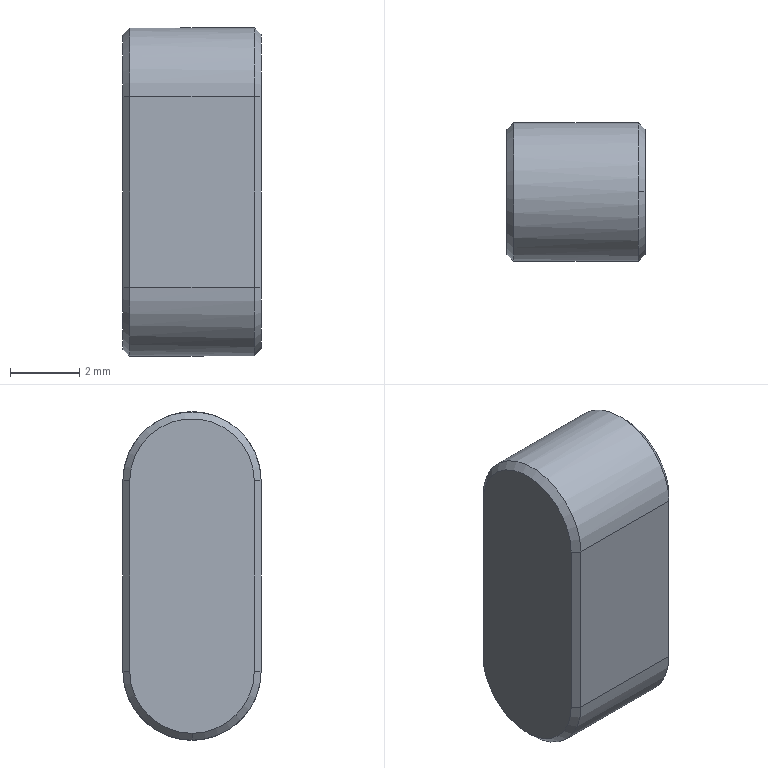Part | STEP file | 02-08 Driving sprocket key | 1 solid | 16 faces | box 4 x 4 x 9.5 mm | volume 137.34 mm3 | plane 8 | cone 6 | cylinder 2 | commonest cylinder face diameters 4 x2
STEP:
#1=CARTESIAN_POINT('',(0.,0.,0.));
#2=DIRECTION('',(0.,0.,1.));
#3=DIRECTION('',(1.,0.,0.));
#4=AXIS2_PLACEMENT_3D('',#1,#2,#3);
#5=CARTESIAN_POINT('',(4.,0.,1.8));
#6=VERTEX_POINT('',#5);
#7=CARTESIAN_POINT('',(4.,-1.8,0.));
#8=VERTEX_POINT('',#7);
#9=CARTESIAN_POINT('',(4.,0.,0.));
#10=DIRECTION('',(1.,0.,0.));
#11=DIRECTION('',(0.,0.,1.));
#12=AXIS2_PLACEMENT_3D('',#9,#10,#11);
#13=CIRCLE('',#12,1.8);
#14=CARTESIAN_POINT('',(4.,0.,0.));
#15=DIRECTION('',(-1.,0.,0.));
#16=DIRECTION('',(0.,0.,1.));
#17=AXIS2_PLACEMENT_3D('',#14,#15,#16);
#18=CONICAL_SURFACE('',#17,1.8,0.7854);
#19=CARTESIAN_POINT('',(6.283,0.));
#20=DIRECTION('',(-1.,0.));
#21=VECTOR('',#20,1.);
#22=LINE('',#19,#21);
#23=(GEOMETRIC_REPRESENTATION_CONTEXT(2)PARAMETRIC_REPRESENTATION_CONTEXT()REPRESENTATION_CONTEXT('',''));
#24=DEFINITIONAL_REPRESENTATION('',(#22),#23);
#25=PCURVE('',#18,#24);
#26=CARTESIAN_POINT('',(4.,-1.8,1.855));
#27=DIRECTION('',(1.,0.,0.));
#28=DIRECTION('',(0.,0.,-1.));
#29=AXIS2_PLACEMENT_3D('',#26,#27,#28);
#30=PLANE('',#29);
#31=CARTESIAN_POINT('',(1.855,1.8));
#32=DIRECTION('',(-1.,0.));
#33=AXIS2_PLACEMENT_2D('',#31,#32);
#34=CIRCLE('',#33,1.8);
#35=(GEOMETRIC_REPRESENTATION_CONTEXT(2)PARAMETRIC_REPRESENTATION_CONTEXT()REPRESENTATION_CONTEXT('',''));
#36=DEFINITIONAL_REPRESENTATION('',(#34),#35);
#37=PCURVE('',#30,#36);
#38=SURFACE_CURVE('',#13,(#25,#37),.PCURVE_S1.);
#39=EDGE_CURVE('',#6,#8,#38,.T.);
#40=ORIENTED_EDGE('',*,*,#39,.F.);
#41=CARTESIAN_POINT('',(3.8,0.,2.));
#42=VERTEX_POINT('',#41);
#43=CARTESIAN_POINT('',(4.,0.,1.8));
#44=DIRECTION('',(-0.7071,0.,0.7071));
#45=VECTOR('',#44,1.);
#46=LINE('',#43,#45);
#47=CARTESIAN_POINT('',(6.283,0.));
#48=DIRECTION('',(0.,1.));
#49=VECTOR('',#48,1.);
#50=LINE('',#47,#49);
#51=(GEOMETRIC_REPRESENTATION_CONTEXT(2)PARAMETRIC_REPRESENTATION_CONTEXT()REPRESENTATION_CONTEXT('',''));
#52=DEFINITIONAL_REPRESENTATION('',(#50),#51);
#53=PCURVE('',#18,#52);
#54=CARTESIAN_POINT('',(4.,0.,0.));
#55=DIRECTION('',(-1.,0.,0.));
#56=DIRECTION('',(0.,0.,1.));
#57=AXIS2_PLACEMENT_3D('',#54,#55,#56);
#58=CONICAL_SURFACE('',#57,1.8,0.7854);
#59=CARTESIAN_POINT('',(0.,0.));
#60=DIRECTION('',(0.,1.));
#61=VECTOR('',#60,1.);
#62=LINE('',#59,#61);
#63=(GEOMETRIC_REPRESENTATION_CONTEXT(2)PARAMETRIC_REPRESENTATION_CONTEXT()REPRESENTATION_CONTEXT('',''));
#64=DEFINITIONAL_REPRESENTATION('',(#62),#63);
#65=PCURVE('',#58,#64);
#66=SURFACE_CURVE('',#46,(#53,#65),.PCURVE_S1.);
#67=EDGE_CURVE('',#6,#42,#66,.T.);
#68=ORIENTED_EDGE('',*,*,#67,.T.);
#69=CARTESIAN_POINT('',(3.8,-2.,0.));
#70=VERTEX_POINT('',#69);
#71=CARTESIAN_POINT('',(3.8,0.,0.));
#72=DIRECTION('',(-1.,0.,0.));
#73=DIRECTION('',(0.,0.,1.));
#74=AXIS2_PLACEMENT_3D('',#71,#72,#73);
#75=CIRCLE('',#74,2.);
#76=CARTESIAN_POINT('',(0.,0.2));
#77=DIRECTION('',(1.,0.));
#78=VECTOR('',#77,1.);
#79=LINE('',#76,#78);
#80=(GEOMETRIC_REPRESENTATION_CONTEXT(2)PARAMETRIC_REPRESENTATION_CONTEXT()REPRESENTATION_CONTEXT('',''));
#81=DEFINITIONAL_REPRESENTATION('',(#79),#80);
#82=PCURVE('',#18,#81);
#83=CARTESIAN_POINT('',(3.8,0.,0.));
#84=DIRECTION('',(-1.,0.,0.));
#85=DIRECTION('',(0.,-1.,0.));
#86=AXIS2_PLACEMENT_3D('',#83,#84,#85);
#87=CYLINDRICAL_SURFACE('',#86,2.);
#88=CARTESIAN_POINT('',(-4.712,0.));
#89=DIRECTION('',(1.,0.));
#90=VECTOR('',#89,1.);
#91=LINE('',#88,#90);
#92=(GEOMETRIC_REPRESENTATION_CONTEXT(2)PARAMETRIC_REPRESENTATION_CONTEXT()REPRESENTATION_CONTEXT('',''));
#93=DEFINITIONAL_REPRESENTATION('',(#91),#92);
#94=PCURVE('',#87,#93);
#95=SURFACE_CURVE('',#75,(#82,#94),.PCURVE_S1.);
#96=EDGE_CURVE('',#70,#42,#95,.T.);
#97=ORIENTED_EDGE('',*,*,#96,.F.);
#98=CARTESIAN_POINT('',(3.9,-1.9,0.));
#99=DIRECTION('',(-0.7071,-0.7071,0.));
#100=VECTOR('',#99,1.);
#101=LINE('',#98,#100);
#102=CARTESIAN_POINT('',(4.712,0.1));
#103=DIRECTION('',(0.,1.));
#104=VECTOR('',#103,1.);
#105=LINE('',#102,#104);
#106=(GEOMETRIC_REPRESENTATION_CONTEXT(2)PARAMETRIC_REPRESENTATION_CONTEXT()REPRESENTATION_CONTEXT('',''));
#107=DEFINITIONAL_REPRESENTATION('',(#105),#106);
#108=PCURVE('',#18,#107);
#109=CARTESIAN_POINT('',(3.8,-2.,-5.5));
#110=DIRECTION('',(0.7071,-0.7071,0.));
#111=DIRECTION('',(0.7071,0.7071,0.));
#112=AXIS2_PLACEMENT_3D('',#109,#110,#111);
#113=PLANE('',#112);
#114=CARTESIAN_POINT('',(0.1414,5.5));
#115=DIRECTION('',(-1.,0.));
#116=VECTOR('',#115,1.);
#117=LINE('',#114,#116);
#118=(GEOMETRIC_REPRESENTATION_CONTEXT(2)PARAMETRIC_REPRESENTATION_CONTEXT()REPRESENTATION_CONTEXT('',''));
#119=DEFINITIONAL_REPRESENTATION('',(#117),#118);
#120=PCURVE('',#113,#119);
#121=SURFACE_CURVE('',#101,(#108,#120),.PCURVE_S1.);
#122=EDGE_CURVE('',#8,#70,#121,.T.);
#123=ORIENTED_EDGE('',*,*,#122,.F.);
#124=EDGE_LOOP('',(#40,#68,#97,#123));
#125=FACE_BOUND('',#124,.T.);
#126=ADVANCED_FACE('',(#125),#18,.T.);
#127=CARTESIAN_POINT('',(0.,-1.8,-5.5));
#128=VERTEX_POINT('',#127);
#129=CARTESIAN_POINT('',(0.,0.,-7.3));
#130=VERTEX_POINT('',#129);
#131=CARTESIAN_POINT('',(0.,0.,-5.5));
#132=DIRECTION('',(1.,0.,0.));
#133=DIRECTION('',(0.,0.,-1.));
#134=AXIS2_PLACEMENT_3D('',#131,#132,#133);
#135=CIRCLE('',#134,1.8);
#136=CARTESIAN_POINT('',(0.,0.,-5.5));
#137=DIRECTION('',(1.,0.,0.));
#138=DIRECTION('',(0.,0.,-1.));
#139=AXIS2_PLACEMENT_3D('',#136,#137,#138);
#140=CONICAL_SURFACE('',#139,1.8,0.7854);
#141=CARTESIAN_POINT('',(0.,0.));
#142=DIRECTION('',(1.,0.));
#143=VECTOR('',#142,1.);
#144=LINE('',#141,#143);
#145=(GEOMETRIC_REPRESENTATION_CONTEXT(2)PARAMETRIC_REPRESENTATION_CONTEXT()REPRESENTATION_CONTEXT('',''));
#146=DEFINITIONAL_REPRESENTATION('',(#144),#145);
#147=PCURVE('',#140,#146);
#148=CARTESIAN_POINT('',(0.,-1.8,1.855));
#149=DIRECTION('',(1.,0.,0.));
#150=DIRECTION('',(0.,0.,-1.));
#151=AXIS2_PLACEMENT_3D('',#148,#149,#150);
#152=PLANE('',#151);
#153=CARTESIAN_POINT('',(7.355,1.8));
#154=DIRECTION('',(1.,0.));
#155=AXIS2_PLACEMENT_2D('',#153,#154);
#156=CIRCLE('',#155,1.8);
#157=(GEOMETRIC_REPRESENTATION_CONTEXT(2)PARAMETRIC_REPRESENTATION_CONTEXT()REPRESENTATION_CONTEXT('',''));
#158=DEFINITIONAL_REPRESENTATION('',(#156),#157);
#159=PCURVE('',#152,#158);
#160=SURFACE_CURVE('',#135,(#147,#159),.PCURVE_S1.);
#161=EDGE_CURVE('',#128,#130,#160,.T.);
#162=ORIENTED_EDGE('',*,*,#161,.T.);
#163=CARTESIAN_POINT('',(0.2,0.,-7.5));
#164=VERTEX_POINT('',#163);
#165=CARTESIAN_POINT('',(0.,0.,-7.3));
#166=DIRECTION('',(0.7071,0.,-0.7071));
#167=VECTOR('',#166,1.);
#168=LINE('',#165,#167);
#169=CARTESIAN_POINT('',(6.283,0.));
#170=DIRECTION('',(0.,1.));
#171=VECTOR('',#170,1.);
#172=LINE('',#169,#171);
#173=(GEOMETRIC_REPRESENTATION_CONTEXT(2)PARAMETRIC_REPRESENTATION_CONTEXT()REPRESENTATION_CONTEXT('',''));
#174=DEFINITIONAL_REPRESENTATION('',(#172),#173);
#175=PCURVE('',#140,#174);
#176=CARTESIAN_POINT('',(0.,0.,-5.5));
#177=DIRECTION('',(1.,0.,0.));
#178=DIRECTION('',(0.,0.,-1.));
#179=AXIS2_PLACEMENT_3D('',#176,#177,#178);
#180=CONICAL_SURFACE('',#179,1.8,0.7854);
#181=CARTESIAN_POINT('',(0.,0.));
#182=DIRECTION('',(0.,1.));
#183=VECTOR('',#182,1.);
#184=LINE('',#181,#183);
#185=(GEOMETRIC_REPRESENTATION_CONTEXT(2)PARAMETRIC_REPRESENTATION_CONTEXT()REPRESENTATION_CONTEXT('',''));
#186=DEFINITIONAL_REPRESENTATION('',(#184),#185);
#187=PCURVE('',#180,#186);
#188=SURFACE_CURVE('',#168,(#175,#187),.PCURVE_S1.);
#189=EDGE_CURVE('',#130,#164,#188,.T.);
#190=ORIENTED_EDGE('',*,*,#189,.T.);
#191=CARTESIAN_POINT('',(0.2,-2.,-5.5));
#192=VERTEX_POINT('',#191);
#193=CARTESIAN_POINT('',(0.2,0.,-5.5));
#194=DIRECTION('',(-1.,0.,0.));
#195=DIRECTION('',(0.,0.,1.));
#196=AXIS2_PLACEMENT_3D('',#193,#194,#195);
#197=CIRCLE('',#196,2.);
#198=CARTESIAN_POINT('',(9.425,0.2));
#199=DIRECTION('',(-1.,0.));
#200=VECTOR('',#199,1.);
#201=LINE('',#198,#200);
#202=(GEOMETRIC_REPRESENTATION_CONTEXT(2)PARAMETRIC_REPRESENTATION_CONTEXT()REPRESENTATION_CONTEXT('',''));
#203=DEFINITIONAL_REPRESENTATION('',(#201),#202);
#204=PCURVE('',#140,#203);
#205=CARTESIAN_POINT('',(3.8,0.,-5.5));
#206=DIRECTION('',(-1.,0.,0.));
#207=DIRECTION('',(0.,-1.,0.));
#208=AXIS2_PLACEMENT_3D('',#205,#206,#207);
#209=CYLINDRICAL_SURFACE('',#208,2.);
#210=CARTESIAN_POINT('',(1.571,3.6));
#211=DIRECTION('',(1.,0.));
#212=VECTOR('',#211,1.);
#213=LINE('',#210,#212);
#214=(GEOMETRIC_REPRESENTATION_CONTEXT(2)PARAMETRIC_REPRESENTATION_CONTEXT()REPRESENTATION_CONTEXT('',''));
#215=DEFINITIONAL_REPRESENTATION('',(#213),#214);
#216=PCURVE('',#209,#215);
#217=SURFACE_CURVE('',#197,(#204,#216),.PCURVE_S1.);
#218=EDGE_CURVE('',#164,#192,#217,.T.);
#219=ORIENTED_EDGE('',*,*,#218,.T.);
#220=CARTESIAN_POINT('',(0.1,-1.9,-5.5));
#221=DIRECTION('',(-0.7071,0.7071,0.));
#222=VECTOR('',#221,1.);
#223=LINE('',#220,#222);
#224=CARTESIAN_POINT('',(4.712,0.1));
#225=DIRECTION('',(0.,-1.));
#226=VECTOR('',#225,1.);
#227=LINE('',#224,#226);
#228=(GEOMETRIC_REPRESENTATION_CONTEXT(2)PARAMETRIC_REPRESENTATION_CONTEXT()REPRESENTATION_CONTEXT('',''));
#229=DEFINITIONAL_REPRESENTATION('',(#227),#228);
#230=PCURVE('',#140,#229);
#231=CARTESIAN_POINT('',(0.2,-2.,-5.5));
#232=DIRECTION('',(0.7071,0.7071,0.));
#233=DIRECTION('',(-0.7071,0.7071,0.));
#234=AXIS2_PLACEMENT_3D('',#231,#232,#233);
#235=PLANE('',#234);
#236=CARTESIAN_POINT('',(0.1414,0.));
#237=DIRECTION('',(1.,0.));
#238=VECTOR('',#237,1.);
#239=LINE('',#236,#238);
#240=(GEOMETRIC_REPRESENTATION_CONTEXT(2)PARAMETRIC_REPRESENTATION_CONTEXT()REPRESENTATION_CONTEXT('',''));
#241=DEFINITIONAL_REPRESENTATION('',(#239),#240);
#242=PCURVE('',#235,#241);
#243=SURFACE_CURVE('',#223,(#230,#242),.PCURVE_S1.);
#244=EDGE_CURVE('',#192,#128,#243,.T.);
#245=ORIENTED_EDGE('',*,*,#244,.T.);
#246=EDGE_LOOP('',(#162,#190,#219,#245));
#247=FACE_BOUND('',#246,.T.);
#248=ADVANCED_FACE('',(#247),#140,.T.);
#249=ORIENTED_EDGE('',*,*,#67,.F.);
#250=CARTESIAN_POINT('',(4.,1.8,0.));
#251=VERTEX_POINT('',#250);
#252=CARTESIAN_POINT('',(4.,0.,0.));
#253=DIRECTION('',(1.,0.,0.));
#254=DIRECTION('',(0.,0.,1.));
#255=AXIS2_PLACEMENT_3D('',#252,#253,#254);
#256=CIRCLE('',#255,1.8);
#257=CARTESIAN_POINT('',(6.283,0.));
#258=DIRECTION('',(-1.,0.));
#259=VECTOR('',#258,1.);
#260=LINE('',#257,#259);
#261=(GEOMETRIC_REPRESENTATION_CONTEXT(2)PARAMETRIC_REPRESENTATION_CONTEXT()REPRESENTATION_CONTEXT('',''));
#262=DEFINITIONAL_REPRESENTATION('',(#260),#261);
#263=PCURVE('',#58,#262);
#264=CARTESIAN_POINT('',(1.855,1.8));
#265=DIRECTION('',(-1.,0.));
#266=AXIS2_PLACEMENT_2D('',#264,#265);
#267=CIRCLE('',#266,1.8);
#268=(GEOMETRIC_REPRESENTATION_CONTEXT(2)PARAMETRIC_REPRESENTATION_CONTEXT()REPRESENTATION_CONTEXT('',''));
#269=DEFINITIONAL_REPRESENTATION('',(#267),#268);
#270=PCURVE('',#30,#269);
#271=SURFACE_CURVE('',#256,(#263,#270),.PCURVE_S1.);
#272=EDGE_CURVE('',#251,#6,#271,.T.);
#273=ORIENTED_EDGE('',*,*,#272,.F.);
#274=CARTESIAN_POINT('',(3.8,2.,0.));
#275=VERTEX_POINT('',#274);
#276=CARTESIAN_POINT('',(3.9,1.9,0.));
#277=DIRECTION('',(0.7071,-0.7071,0.));
#278=VECTOR('',#277,1.);
#279=LINE('',#276,#278);
#280=CARTESIAN_POINT('',(1.571,0.1));
#281=DIRECTION('',(0.,-1.));
#282=VECTOR('',#281,1.);
#283=LINE('',#280,#282);
#284=(GEOMETRIC_REPRESENTATION_CONTEXT(2)PARAMETRIC_REPRESENTATION_CONTEXT()REPRESENTATION_CONTEXT('',''));
#285=DEFINITIONAL_REPRESENTATION('',(#283),#284);
#286=PCURVE('',#58,#285);
#287=CARTESIAN_POINT('',(4.,1.8,-5.5));
#288=DIRECTION('',(0.7071,0.7071,0.));
#289=DIRECTION('',(-0.7071,0.7071,0.));
#290=AXIS2_PLACEMENT_3D('',#287,#288,#289);
#291=PLANE('',#290);
#292=CARTESIAN_POINT('',(0.1414,5.5));
#293=DIRECTION('',(-1.,0.));
#294=VECTOR('',#293,1.);
#295=LINE('',#292,#294);
#296=(GEOMETRIC_REPRESENTATION_CONTEXT(2)PARAMETRIC_REPRESENTATION_CONTEXT()REPRESENTATION_CONTEXT('',''));
#297=DEFINITIONAL_REPRESENTATION('',(#295),#296);
#298=PCURVE('',#291,#297);
#299=SURFACE_CURVE('',#279,(#286,#298),.PCURVE_S1.);
#300=EDGE_CURVE('',#275,#251,#299,.T.);
#301=ORIENTED_EDGE('',*,*,#300,.F.);
#302=CARTESIAN_POINT('',(3.8,0.,0.));
#303=DIRECTION('',(-1.,0.,0.));
#304=DIRECTION('',(0.,0.,1.));
#305=AXIS2_PLACEMENT_3D('',#302,#303,#304);
#306=CIRCLE('',#305,2.);
#307=CARTESIAN_POINT('',(0.,0.2));
#308=DIRECTION('',(1.,0.));
#309=VECTOR('',#308,1.);
#310=LINE('',#307,#309);
#311=(GEOMETRIC_REPRESENTATION_CONTEXT(2)PARAMETRIC_REPRESENTATION_CONTEXT()REPRESENTATION_CONTEXT('',''));
#312=DEFINITIONAL_REPRESENTATION('',(#310),#311);
#313=PCURVE('',#58,#312);
#314=CARTESIAN_POINT('',(1.571,0.));
#315=DIRECTION('',(1.,0.));
#316=VECTOR('',#315,1.);
#317=LINE('',#314,#316);
#318=(GEOMETRIC_REPRESENTATION_CONTEXT(2)PARAMETRIC_REPRESENTATION_CONTEXT()REPRESENTATION_CONTEXT('',''));
#319=DEFINITIONAL_REPRESENTATION('',(#317),#318);
#320=PCURVE('',#87,#319);
#321=SURFACE_CURVE('',#306,(#313,#320),.PCURVE_S1.);
#322=EDGE_CURVE('',#42,#275,#321,.T.);
#323=ORIENTED_EDGE('',*,*,#322,.F.);
#324=EDGE_LOOP('',(#249,#273,#301,#323));
#325=FACE_BOUND('',#324,.T.);
#326=ADVANCED_FACE('',(#325),#58,.T.);
#327=CARTESIAN_POINT('',(4.,-1.8,-5.5));
#328=VERTEX_POINT('',#327);
#329=CARTESIAN_POINT('',(4.,1.8,-5.5));
#330=VERTEX_POINT('',#329);
#331=CARTESIAN_POINT('',(4.,0.,-5.5));
#332=DIRECTION('',(1.,0.,0.));
#333=DIRECTION('',(0.,0.,1.));
#334=AXIS2_PLACEMENT_3D('',#331,#332,#333);
#335=CIRCLE('',#334,1.8);
#336=CARTESIAN_POINT('',(7.355,1.8));
#337=DIRECTION('',(-1.,0.));
#338=AXIS2_PLACEMENT_2D('',#336,#337);
#339=CIRCLE('',#338,1.8);
#340=(GEOMETRIC_REPRESENTATION_CONTEXT(2)PARAMETRIC_REPRESENTATION_CONTEXT()REPRESENTATION_CONTEXT('',''));
#341=DEFINITIONAL_REPRESENTATION('',(#339),#340);
#342=PCURVE('',#30,#341);
#343=CARTESIAN_POINT('',(4.,0.,-5.5));
#344=DIRECTION('',(-1.,0.,0.));
#345=DIRECTION('',(0.,0.,1.));
#346=AXIS2_PLACEMENT_3D('',#343,#344,#345);
#347=CONICAL_SURFACE('',#346,1.8,0.7854);
#348=CARTESIAN_POINT('',(6.283,0.));
#349=DIRECTION('',(-1.,0.));
#350=VECTOR('',#349,1.);
#351=LINE('',#348,#350);
#352=(GEOMETRIC_REPRESENTATION_CONTEXT(2)PARAMETRIC_REPRESENTATION_CONTEXT()REPRESENTATION_CONTEXT('',''));
#353=DEFINITIONAL_REPRESENTATION('',(#351),#352);
#354=PCURVE('',#347,#353);
#355=SURFACE_CURVE('',#335,(#342,#354),.PCURVE_S1.);
#356=EDGE_CURVE('',#328,#330,#355,.T.);
#357=ORIENTED_EDGE('',*,*,#356,.T.);
#358=CARTESIAN_POINT('',(4.,1.8,-2.75));
#359=DIRECTION('',(0.,0.,1.));
#360=VECTOR('',#359,1.);
#361=LINE('',#358,#360);
#362=CARTESIAN_POINT('',(4.605,3.6));
#363=DIRECTION('',(-1.,0.));
#364=VECTOR('',#363,1.);
#365=LINE('',#362,#364);
#366=(GEOMETRIC_REPRESENTATION_CONTEXT(2)PARAMETRIC_REPRESENTATION_CONTEXT()REPRESENTATION_CONTEXT('',''));
#367=DEFINITIONAL_REPRESENTATION('',(#365),#366);
#368=PCURVE('',#30,#367);
#369=CARTESIAN_POINT('',(0.,2.75));
#370=DIRECTION('',(0.,1.));
#371=VECTOR('',#370,1.);
#372=LINE('',#369,#371);
#373=(GEOMETRIC_REPRESENTATION_CONTEXT(2)PARAMETRIC_REPRESENTATION_CONTEXT()REPRESENTATION_CONTEXT('',''));
#374=DEFINITIONAL_REPRESENTATION('',(#372),#373);
#375=PCURVE('',#291,#374);
#376=SURFACE_CURVE('',#361,(#368,#375),.PCURVE_S1.);
#377=EDGE_CURVE('',#330,#251,#376,.T.);
#378=ORIENTED_EDGE('',*,*,#377,.T.);
#379=ORIENTED_EDGE('',*,*,#272,.T.);
#380=ORIENTED_EDGE('',*,*,#39,.T.);
#381=CARTESIAN_POINT('',(4.,-1.8,-2.75));
#382=DIRECTION('',(0.,0.,-1.));
#383=VECTOR('',#382,1.);
#384=LINE('',#381,#383);
#385=CARTESIAN_POINT('',(4.605,0.));
#386=DIRECTION('',(1.,0.));
#387=VECTOR('',#386,1.);
#388=LINE('',#385,#387);
#389=(GEOMETRIC_REPRESENTATION_CONTEXT(2)PARAMETRIC_REPRESENTATION_CONTEXT()REPRESENTATION_CONTEXT('',''));
#390=DEFINITIONAL_REPRESENTATION('',(#388),#389);
#391=PCURVE('',#30,#390);
#392=CARTESIAN_POINT('',(0.2828,2.75));
#393=DIRECTION('',(0.,-1.));
#394=VECTOR('',#393,1.);
#395=LINE('',#392,#394);
#396=(GEOMETRIC_REPRESENTATION_CONTEXT(2)PARAMETRIC_REPRESENTATION_CONTEXT()REPRESENTATION_CONTEXT('',''));
#397=DEFINITIONAL_REPRESENTATION('',(#395),#396);
#398=PCURVE('',#113,#397);
#399=SURFACE_CURVE('',#384,(#391,#398),.PCURVE_S1.);
#400=EDGE_CURVE('',#8,#328,#399,.T.);
#401=ORIENTED_EDGE('',*,*,#400,.T.);
#402=EDGE_LOOP('',(#357,#378,#379,#380,#401));
#403=FACE_BOUND('',#402,.T.);
#404=ADVANCED_FACE('',(#403),#30,.T.);
#405=ORIENTED_EDGE('',*,*,#96,.T.);
#406=ORIENTED_EDGE('',*,*,#322,.T.);
#407=CARTESIAN_POINT('',(0.2,2.,0.));
#408=VERTEX_POINT('',#407);
#409=CARTESIAN_POINT('',(2.,2.,0.));
#410=DIRECTION('',(1.,0.,0.));
#411=VECTOR('',#410,1.);
#412=LINE('',#409,#411);
#413=CARTESIAN_POINT('',(3.142,1.8));
#414=DIRECTION('',(0.,-1.));
#415=VECTOR('',#414,1.);
#416=LINE('',#413,#415);
#417=(GEOMETRIC_REPRESENTATION_CONTEXT(2)PARAMETRIC_REPRESENTATION_CONTEXT()REPRESENTATION_CONTEXT('',''));
#418=DEFINITIONAL_REPRESENTATION('',(#416),#417);
#419=PCURVE('',#87,#418);
#420=CARTESIAN_POINT('',(0.2,2.,0.));
#421=DIRECTION('',(0.,-1.,0.));
#422=DIRECTION('',(0.,0.,-1.));
#423=AXIS2_PLACEMENT_3D('',#420,#421,#422);
#424=PLANE('',#423);
#425=CARTESIAN_POINT('',(0.,1.8));
#426=DIRECTION('',(0.,1.));
#427=VECTOR('',#426,1.);
#428=LINE('',#425,#427);
#429=(GEOMETRIC_REPRESENTATION_CONTEXT(2)PARAMETRIC_REPRESENTATION_CONTEXT()REPRESENTATION_CONTEXT('',''));
#430=DEFINITIONAL_REPRESENTATION('',(#428),#429);
#431=PCURVE('',#424,#430);
#432=SURFACE_CURVE('',#412,(#419,#431),.PCURVE_S1.);
#433=EDGE_CURVE('',#408,#275,#432,.T.);
#434=ORIENTED_EDGE('',*,*,#433,.F.);
#435=CARTESIAN_POINT('',(0.2,-2.,0.));
#436=VERTEX_POINT('',#435);
#437=CARTESIAN_POINT('',(0.2,0.,0.));
#438=DIRECTION('',(-1.,0.,0.));
#439=DIRECTION('',(0.,0.,1.));
#440=AXIS2_PLACEMENT_3D('',#437,#438,#439);
#441=CIRCLE('',#440,2.);
#442=CARTESIAN_POINT('',(-4.712,3.6));
#443=DIRECTION('',(1.,0.));
#444=VECTOR('',#443,1.);
#445=LINE('',#442,#444);
#446=(GEOMETRIC_REPRESENTATION_CONTEXT(2)PARAMETRIC_REPRESENTATION_CONTEXT()REPRESENTATION_CONTEXT('',''));
#447=DEFINITIONAL_REPRESENTATION('',(#445),#446);
#448=PCURVE('',#87,#447);
#449=CARTESIAN_POINT('',(0.,0.,0.));
#450=DIRECTION('',(1.,0.,0.));
#451=DIRECTION('',(0.,0.,-1.));
#452=AXIS2_PLACEMENT_3D('',#449,#450,#451);
#453=CONICAL_SURFACE('',#452,1.8,0.7854);
#454=CARTESIAN_POINT('',(9.425,0.2));
#455=DIRECTION('',(-1.,0.));
#456=VECTOR('',#455,1.);
#457=LINE('',#454,#456);
#458=(GEOMETRIC_REPRESENTATION_CONTEXT(2)PARAMETRIC_REPRESENTATION_CONTEXT()REPRESENTATION_CONTEXT('',''));
#459=DEFINITIONAL_REPRESENTATION('',(#457),#458);
#460=PCURVE('',#453,#459);
#461=SURFACE_CURVE('',#441,(#448,#460),.PCURVE_S1.);
#462=EDGE_CURVE('',#436,#408,#461,.T.);
#463=ORIENTED_EDGE('',*,*,#462,.F.);
#464=CARTESIAN_POINT('',(2.,-2.,-0.000000001));
#465=DIRECTION('',(-1.,0.,0.));
#466=VECTOR('',#465,1.);
#467=LINE('',#464,#466);
#468=CARTESIAN_POINT('',(0.,1.8));
#469=DIRECTION('',(0.,1.));
#470=VECTOR('',#469,1.);
#471=LINE('',#468,#470);
#472=(GEOMETRIC_REPRESENTATION_CONTEXT(2)PARAMETRIC_REPRESENTATION_CONTEXT()REPRESENTATION_CONTEXT('',''));
#473=DEFINITIONAL_REPRESENTATION('',(#471),#472);
#474=PCURVE('',#87,#473);
#475=CARTESIAN_POINT('',(0.2,-2.,-5.5));
#476=DIRECTION('',(0.,1.,0.));
#477=DIRECTION('',(0.,0.,1.));
#478=AXIS2_PLACEMENT_3D('',#475,#476,#477);
#479=PLANE('',#478);
#480=CARTESIAN_POINT('',(5.5,1.8));
#481=DIRECTION('',(0.,-1.));
#482=VECTOR('',#481,1.);
#483=LINE('',#480,#482);
#484=(GEOMETRIC_REPRESENTATION_CONTEXT(2)PARAMETRIC_REPRESENTATION_CONTEXT()REPRESENTATION_CONTEXT('',''));
#485=DEFINITIONAL_REPRESENTATION('',(#483),#484);
#486=PCURVE('',#479,#485);
#487=SURFACE_CURVE('',#467,(#474,#486),.PCURVE_S1.);
#488=EDGE_CURVE('',#70,#436,#487,.T.);
#489=ORIENTED_EDGE('',*,*,#488,.F.);
#490=EDGE_LOOP('',(#405,#406,#434,#463,#489));
#491=FACE_BOUND('',#490,.T.);
#492=ADVANCED_FACE('',(#491),#87,.T.);
#493=ORIENTED_EDGE('',*,*,#300,.T.);
#494=ORIENTED_EDGE('',*,*,#377,.F.);
#495=CARTESIAN_POINT('',(3.8,2.,-5.5));
#496=VERTEX_POINT('',#495);
#497=CARTESIAN_POINT('',(3.9,1.9,-5.5));
#498=DIRECTION('',(-0.7071,0.7071,0.));
#499=VECTOR('',#498,1.);
#500=LINE('',#497,#499);
#501=CARTESIAN_POINT('',(0.1414,0.));
#502=DIRECTION('',(1.,0.));
#503=VECTOR('',#502,1.);
#504=LINE('',#501,#503);
#505=(GEOMETRIC_REPRESENTATION_CONTEXT(2)PARAMETRIC_REPRESENTATION_CONTEXT()REPRESENTATION_CONTEXT('',''));
#506=DEFINITIONAL_REPRESENTATION('',(#504),#505);
#507=PCURVE('',#291,#506);
#508=CARTESIAN_POINT('',(1.571,0.1));
#509=DIRECTION('',(0.,1.));
#510=VECTOR('',#509,1.);
#511=LINE('',#508,#510);
#512=(GEOMETRIC_REPRESENTATION_CONTEXT(2)PARAMETRIC_REPRESENTATION_CONTEXT()REPRESENTATION_CONTEXT('',''));
#513=DEFINITIONAL_REPRESENTATION('',(#511),#512);
#514=PCURVE('',#347,#513);
#515=SURFACE_CURVE('',#500,(#507,#514),.PCURVE_S1.);
#516=EDGE_CURVE('',#330,#496,#515,.T.);
#517=ORIENTED_EDGE('',*,*,#516,.T.);
#518=CARTESIAN_POINT('',(3.8,2.,-2.75));
#519=DIRECTION('',(0.,0.,1.));
#520=VECTOR('',#519,1.);
#521=LINE('',#518,#520);
#522=CARTESIAN_POINT('',(0.2828,2.75));
#523=DIRECTION('',(0.,1.));
#524=VECTOR('',#523,1.);
#525=LINE('',#522,#524);
#526=(GEOMETRIC_REPRESENTATION_CONTEXT(2)PARAMETRIC_REPRESENTATION_CONTEXT()REPRESENTATION_CONTEXT('',''));
#527=DEFINITIONAL_REPRESENTATION('',(#525),#526);
#528=PCURVE('',#291,#527);
#529=CARTESIAN_POINT('',(2.75,3.6));
#530=DIRECTION('',(-1.,0.));
#531=VECTOR('',#530,1.);
#532=LINE('',#529,#531);
#533=(GEOMETRIC_REPRESENTATION_CONTEXT(2)PARAMETRIC_REPRESENTATION_CONTEXT()REPRESENTATION_CONTEXT('',''));
#534=DEFINITIONAL_REPRESENTATION('',(#532),#533);
#535=PCURVE('',#424,#534);
#536=SURFACE_CURVE('',#521,(#528,#535),.PCURVE_S1.);
#537=EDGE_CURVE('',#496,#275,#536,.T.);
#538=ORIENTED_EDGE('',*,*,#537,.T.);
#539=EDGE_LOOP('',(#493,#494,#517,#538));
#540=FACE_BOUND('',#539,.T.);
#541=ADVANCED_FACE('',(#540),#291,.T.);
#542=ORIENTED_EDGE('',*,*,#356,.F.);
#543=CARTESIAN_POINT('',(3.8,-2.,-5.5));
#544=VERTEX_POINT('',#543);
#545=CARTESIAN_POINT('',(3.9,-1.9,-5.5));
#546=DIRECTION('',(0.7071,0.7071,0.));
#547=VECTOR('',#546,1.);
#548=LINE('',#545,#547);
#549=CARTESIAN_POINT('',(4.712,0.1));
#550=DIRECTION('',(0.,-1.));
#551=VECTOR('',#550,1.);
#552=LINE('',#549,#551);
#553=(GEOMETRIC_REPRESENTATION_CONTEXT(2)PARAMETRIC_REPRESENTATION_CONTEXT()REPRESENTATION_CONTEXT('',''));
#554=DEFINITIONAL_REPRESENTATION('',(#552),#553);
#555=PCURVE('',#347,#554);
#556=CARTESIAN_POINT('',(0.1414,-0.000000001));
#557=DIRECTION('',(1.,0.));
#558=VECTOR('',#557,1.);
#559=LINE('',#556,#558);
#560=(GEOMETRIC_REPRESENTATION_CONTEXT(2)PARAMETRIC_REPRESENTATION_CONTEXT()REPRESENTATION_CONTEXT('',''));
#561=DEFINITIONAL_REPRESENTATION('',(#559),#560);
#562=PCURVE('',#113,#561);
#563=SURFACE_CURVE('',#548,(#555,#562),.PCURVE_S1.);
#564=EDGE_CURVE('',#544,#328,#563,.T.);
#565=ORIENTED_EDGE('',*,*,#564,.F.);
#566=CARTESIAN_POINT('',(3.8,0.,-5.5));
#567=DIRECTION('',(-1.,0.,0.));
#568=DIRECTION('',(0.,0.,1.));
#569=AXIS2_PLACEMENT_3D('',#566,#567,#568);
#570=CIRCLE('',#569,2.);
#571=CARTESIAN_POINT('',(0.,0.2));
#572=DIRECTION('',(1.,0.));
#573=VECTOR('',#572,1.);
#574=LINE('',#571,#573);
#575=(GEOMETRIC_REPRESENTATION_CONTEXT(2)PARAMETRIC_REPRESENTATION_CONTEXT()REPRESENTATION_CONTEXT('',''));
#576=DEFINITIONAL_REPRESENTATION('',(#574),#575);
#577=PCURVE('',#347,#576);
#578=CARTESIAN_POINT('',(1.571,0.));
#579=DIRECTION('',(1.,0.));
#580=VECTOR('',#579,1.);
#581=LINE('',#578,#580);
#582=(GEOMETRIC_REPRESENTATION_CONTEXT(2)PARAMETRIC_REPRESENTATION_CONTEXT()REPRESENTATION_CONTEXT('',''));
#583=DEFINITIONAL_REPRESENTATION('',(#581),#582);
#584=PCURVE('',#209,#583);
#585=SURFACE_CURVE('',#570,(#577,#584),.PCURVE_S1.);
#586=EDGE_CURVE('',#496,#544,#585,.T.);
#587=ORIENTED_EDGE('',*,*,#586,.F.);
#588=ORIENTED_EDGE('',*,*,#516,.F.);
#589=EDGE_LOOP('',(#542,#565,#587,#588));
#590=FACE_BOUND('',#589,.T.);
#591=ADVANCED_FACE('',(#590),#347,.T.);
#592=ORIENTED_EDGE('',*,*,#564,.T.);
#593=ORIENTED_EDGE('',*,*,#400,.F.);
#594=ORIENTED_EDGE('',*,*,#122,.T.);
#595=CARTESIAN_POINT('',(3.8,-2.,-2.75));
#596=DIRECTION('',(0.,0.,-1.));
#597=VECTOR('',#596,1.);
#598=LINE('',#595,#597);
#599=CARTESIAN_POINT('',(0.,2.75));
#600=DIRECTION('',(0.,-1.));
#601=VECTOR('',#600,1.);
#602=LINE('',#599,#601);
#603=(GEOMETRIC_REPRESENTATION_CONTEXT(2)PARAMETRIC_REPRESENTATION_CONTEXT()REPRESENTATION_CONTEXT('',''));
#604=DEFINITIONAL_REPRESENTATION('',(#602),#603);
#605=PCURVE('',#113,#604);
#606=CARTESIAN_POINT('',(2.75,3.6));
#607=DIRECTION('',(-1.,0.));
#608=VECTOR('',#607,1.);
#609=LINE('',#606,#608);
#610=(GEOMETRIC_REPRESENTATION_CONTEXT(2)PARAMETRIC_REPRESENTATION_CONTEXT()REPRESENTATION_CONTEXT('',''));
#611=DEFINITIONAL_REPRESENTATION('',(#609),#610);
#612=PCURVE('',#479,#611);
#613=SURFACE_CURVE('',#598,(#605,#612),.PCURVE_S1.);
#614=EDGE_CURVE('',#70,#544,#613,.T.);
#615=ORIENTED_EDGE('',*,*,#614,.T.);
#616=EDGE_LOOP('',(#592,#593,#594,#615));
#617=FACE_BOUND('',#616,.T.);
#618=ADVANCED_FACE('',(#617),#113,.T.);
#619=CARTESIAN_POINT('',(0.,-1.8,0.));
#620=VERTEX_POINT('',#619);
#621=CARTESIAN_POINT('',(0.,1.8,0.));
#622=VERTEX_POINT('',#621);
#623=CARTESIAN_POINT('',(0.,0.,0.));
#624=DIRECTION('',(-1.,0.,0.));
#625=DIRECTION('',(0.,0.,-1.));
#626=AXIS2_PLACEMENT_3D('',#623,#624,#625);
#627=CIRCLE('',#626,1.8);
#628=CARTESIAN_POINT('',(6.283,0.));
#629=DIRECTION('',(-1.,0.));
#630=VECTOR('',#629,1.);
#631=LINE('',#628,#630);
#632=(GEOMETRIC_REPRESENTATION_CONTEXT(2)PARAMETRIC_REPRESENTATION_CONTEXT()REPRESENTATION_CONTEXT('',''));
#633=DEFINITIONAL_REPRESENTATION('',(#631),#632);
#634=PCURVE('',#453,#633);
#635=CARTESIAN_POINT('',(3.655,1.8));
#636=CARTESIAN_POINT('',(3.655,-1.318));
#637=CARTESIAN_POINT('',(0.9546,0.2412));
#638=CARTESIAN_POINT('',(-1.745,1.8));
#639=CARTESIAN_POINT('',(0.9546,3.359));
#640=CARTESIAN_POINT('',(3.655,4.918));
#641=CARTESIAN_POINT('',(3.655,1.8));
#642=(BOUNDED_CURVE()B_SPLINE_CURVE(2,(#635,#636,#637,#638,#639,#640,#641),.UNSPECIFIED.,.T.,.F.)B_SPLINE_CURVE_WITH_KNOTS((1,2,2,2,2,1),(-2.094,0.,2.094,4.189,6.283,8.378),.UNSPECIFIED.)CURVE()GEOMETRIC_REPRESENTATION_ITEM()RATIONAL_B_SPLINE_CURVE((1.,0.5,1.,0.5,1.,0.5,1.))REPRESENTATION_ITEM(''));
#643=(GEOMETRIC_REPRESENTATION_CONTEXT(2)PARAMETRIC_REPRESENTATION_CONTEXT()REPRESENTATION_CONTEXT('',''));
#644=DEFINITIONAL_REPRESENTATION('',(#642),#643);
#645=PCURVE('',#152,#644);
#646=SURFACE_CURVE('',#627,(#634,#645),.PCURVE_S1.);
#647=EDGE_CURVE('',#620,#622,#646,.T.);
#648=ORIENTED_EDGE('',*,*,#647,.F.);
#649=CARTESIAN_POINT('',(0.1,-1.9,0.));
#650=DIRECTION('',(0.7071,-0.7071,0.));
#651=VECTOR('',#650,1.);
#652=LINE('',#649,#651);
#653=CARTESIAN_POINT('',(4.712,0.1));
#654=DIRECTION('',(0.,1.));
#655=VECTOR('',#654,1.);
#656=LINE('',#653,#655);
#657=(GEOMETRIC_REPRESENTATION_CONTEXT(2)PARAMETRIC_REPRESENTATION_CONTEXT()REPRESENTATION_CONTEXT('',''));
#658=DEFINITIONAL_REPRESENTATION('',(#656),#657);
#659=PCURVE('',#453,#658);
#660=CARTESIAN_POINT('',(0.1414,5.5));
#661=DIRECTION('',(-1.,0.));
#662=VECTOR('',#661,1.);
#663=LINE('',#660,#662);
#664=(GEOMETRIC_REPRESENTATION_CONTEXT(2)PARAMETRIC_REPRESENTATION_CONTEXT()REPRESENTATION_CONTEXT('',''));
#665=DEFINITIONAL_REPRESENTATION('',(#663),#664);
#666=PCURVE('',#235,#665);
#667=SURFACE_CURVE('',#652,(#659,#666),.PCURVE_S1.);
#668=EDGE_CURVE('',#620,#436,#667,.T.);
#669=ORIENTED_EDGE('',*,*,#668,.T.);
#670=ORIENTED_EDGE('',*,*,#462,.T.);
#671=CARTESIAN_POINT('',(0.1,1.9,0.));
#672=DIRECTION('',(-0.7071,-0.7071,0.));
#673=VECTOR('',#672,1.);
#674=LINE('',#671,#673);
#675=CARTESIAN_POINT('',(1.571,0.1));
#676=DIRECTION('',(0.,-1.));
#677=VECTOR('',#676,1.);
#678=LINE('',#675,#677);
#679=(GEOMETRIC_REPRESENTATION_CONTEXT(2)PARAMETRIC_REPRESENTATION_CONTEXT()REPRESENTATION_CONTEXT('',''));
#680=DEFINITIONAL_REPRESENTATION('',(#678),#679);
#681=PCURVE('',#453,#680);
#682=CARTESIAN_POINT('',(0.,1.8,-5.5));
#683=DIRECTION('',(0.7071,-0.7071,0.));
#684=DIRECTION('',(0.7071,0.7071,0.));
#685=AXIS2_PLACEMENT_3D('',#682,#683,#684);
#686=PLANE('',#685);
#687=CARTESIAN_POINT('',(0.1414,5.5));
#688=DIRECTION('',(-1.,0.));
#689=VECTOR('',#688,1.);
#690=LINE('',#687,#689);
#691=(GEOMETRIC_REPRESENTATION_CONTEXT(2)PARAMETRIC_REPRESENTATION_CONTEXT()REPRESENTATION_CONTEXT('',''));
#692=DEFINITIONAL_REPRESENTATION('',(#690),#691);
#693=PCURVE('',#686,#692);
#694=SURFACE_CURVE('',#674,(#681,#693),.PCURVE_S1.);
#695=EDGE_CURVE('',#408,#622,#694,.T.);
#696=ORIENTED_EDGE('',*,*,#695,.T.);
#697=EDGE_LOOP('',(#648,#669,#670,#696));
#698=FACE_BOUND('',#697,.T.);
#699=ADVANCED_FACE('',(#698),#453,.T.);
#700=CARTESIAN_POINT('',(0.2,-2.,-2.75));
#701=DIRECTION('',(0.,0.,1.));
#702=VECTOR('',#701,1.);
#703=LINE('',#700,#702);
#704=CARTESIAN_POINT('',(2.75,0.));
#705=DIRECTION('',(1.,0.));
#706=VECTOR('',#705,1.);
#707=LINE('',#704,#706);
#708=(GEOMETRIC_REPRESENTATION_CONTEXT(2)PARAMETRIC_REPRESENTATION_CONTEXT()REPRESENTATION_CONTEXT('',''));
#709=DEFINITIONAL_REPRESENTATION('',(#707),#708);
#710=PCURVE('',#479,#709);
#711=CARTESIAN_POINT('',(0.,2.75));
#712=DIRECTION('',(0.,1.));
#713=VECTOR('',#712,1.);
#714=LINE('',#711,#713);
#715=(GEOMETRIC_REPRESENTATION_CONTEXT(2)PARAMETRIC_REPRESENTATION_CONTEXT()REPRESENTATION_CONTEXT('',''));
#716=DEFINITIONAL_REPRESENTATION('',(#714),#715);
#717=PCURVE('',#235,#716);
#718=SURFACE_CURVE('',#703,(#710,#717),.PCURVE_S1.);
#719=EDGE_CURVE('',#192,#436,#718,.T.);
#720=ORIENTED_EDGE('',*,*,#719,.F.);
#721=CARTESIAN_POINT('',(2.,-2.,-5.5));
#722=DIRECTION('',(-1.,0.,0.));
#723=VECTOR('',#722,1.);
#724=LINE('',#721,#723);
#725=CARTESIAN_POINT('',(0.,1.8));
#726=DIRECTION('',(0.,-1.));
#727=VECTOR('',#726,1.);
#728=LINE('',#725,#727);
#729=(GEOMETRIC_REPRESENTATION_CONTEXT(2)PARAMETRIC_REPRESENTATION_CONTEXT()REPRESENTATION_CONTEXT('',''));
#730=DEFINITIONAL_REPRESENTATION('',(#728),#729);
#731=PCURVE('',#479,#730);
#732=CARTESIAN_POINT('',(6.283,1.8));
#733=DIRECTION('',(0.,1.));
#734=VECTOR('',#733,1.);
#735=LINE('',#732,#734);
#736=(GEOMETRIC_REPRESENTATION_CONTEXT(2)PARAMETRIC_REPRESENTATION_CONTEXT()REPRESENTATION_CONTEXT('',''));
#737=DEFINITIONAL_REPRESENTATION('',(#735),#736);
#738=PCURVE('',#209,#737);
#739=SURFACE_CURVE('',#724,(#731,#738),.PCURVE_S1.);
#740=EDGE_CURVE('',#544,#192,#739,.T.);
#741=ORIENTED_EDGE('',*,*,#740,.F.);
#742=ORIENTED_EDGE('',*,*,#614,.F.);
#743=ORIENTED_EDGE('',*,*,#488,.T.);
#744=EDGE_LOOP('',(#720,#741,#742,#743));
#745=FACE_BOUND('',#744,.T.);
#746=ADVANCED_FACE('',(#745),#479,.F.);
#747=CARTESIAN_POINT('',(0.2,2.,-5.5));
#748=VERTEX_POINT('',#747);
#749=CARTESIAN_POINT('',(0.2,2.,-2.75));
#750=DIRECTION('',(0.,0.,-1.));
#751=VECTOR('',#750,1.);
#752=LINE('',#749,#751);
#753=CARTESIAN_POINT('',(2.75,0.));
#754=DIRECTION('',(1.,0.));
#755=VECTOR('',#754,1.);
#756=LINE('',#753,#755);
#757=(GEOMETRIC_REPRESENTATION_CONTEXT(2)PARAMETRIC_REPRESENTATION_CONTEXT()REPRESENTATION_CONTEXT('',''));
#758=DEFINITIONAL_REPRESENTATION('',(#756),#757);
#759=PCURVE('',#424,#758);
#760=CARTESIAN_POINT('',(0.2828,2.75));
#761=DIRECTION('',(0.,-1.));
#762=VECTOR('',#761,1.);
#763=LINE('',#760,#762);
#764=(GEOMETRIC_REPRESENTATION_CONTEXT(2)PARAMETRIC_REPRESENTATION_CONTEXT()REPRESENTATION_CONTEXT('',''));
#765=DEFINITIONAL_REPRESENTATION('',(#763),#764);
#766=PCURVE('',#686,#765);
#767=SURFACE_CURVE('',#752,(#759,#766),.PCURVE_S1.);
#768=EDGE_CURVE('',#408,#748,#767,.T.);
#769=ORIENTED_EDGE('',*,*,#768,.F.);
#770=ORIENTED_EDGE('',*,*,#433,.T.);
#771=ORIENTED_EDGE('',*,*,#537,.F.);
#772=CARTESIAN_POINT('',(2.,2.,-5.5));
#773=DIRECTION('',(1.,0.,0.));
#774=VECTOR('',#773,1.);
#775=LINE('',#772,#774);
#776=CARTESIAN_POINT('',(5.5,1.8));
#777=DIRECTION('',(0.,1.));
#778=VECTOR('',#777,1.);
#779=LINE('',#776,#778);
#780=(GEOMETRIC_REPRESENTATION_CONTEXT(2)PARAMETRIC_REPRESENTATION_CONTEXT()REPRESENTATION_CONTEXT('',''));
#781=DEFINITIONAL_REPRESENTATION('',(#779),#780);
#782=PCURVE('',#424,#781);
#783=CARTESIAN_POINT('',(3.142,1.8));
#784=DIRECTION('',(0.,-1.));
#785=VECTOR('',#784,1.);
#786=LINE('',#783,#785);
#787=(GEOMETRIC_REPRESENTATION_CONTEXT(2)PARAMETRIC_REPRESENTATION_CONTEXT()REPRESENTATION_CONTEXT('',''));
#788=DEFINITIONAL_REPRESENTATION('',(#786),#787);
#789=PCURVE('',#209,#788);
#790=SURFACE_CURVE('',#775,(#782,#789),.PCURVE_S1.);
#791=EDGE_CURVE('',#748,#496,#790,.T.);
#792=ORIENTED_EDGE('',*,*,#791,.F.);
#793=EDGE_LOOP('',(#769,#770,#771,#792));
#794=FACE_BOUND('',#793,.T.);
#795=ADVANCED_FACE('',(#794),#424,.F.);
#796=CARTESIAN_POINT('',(0.2,0.,-5.5));
#797=DIRECTION('',(-1.,0.,0.));
#798=DIRECTION('',(0.,0.,1.));
#799=AXIS2_PLACEMENT_3D('',#796,#797,#798);
#800=CIRCLE('',#799,2.);
#801=CARTESIAN_POINT('',(1.571,3.6));
#802=DIRECTION('',(1.,0.));
#803=VECTOR('',#802,1.);
#804=LINE('',#801,#803);
#805=(GEOMETRIC_REPRESENTATION_CONTEXT(2)PARAMETRIC_REPRESENTATION_CONTEXT()REPRESENTATION_CONTEXT('',''));
#806=DEFINITIONAL_REPRESENTATION('',(#804),#805);
#807=PCURVE('',#209,#806);
#808=CARTESIAN_POINT('',(3.142,0.2));
#809=DIRECTION('',(-1.,0.));
#810=VECTOR('',#809,1.);
#811=LINE('',#808,#810);
#812=(GEOMETRIC_REPRESENTATION_CONTEXT(2)PARAMETRIC_REPRESENTATION_CONTEXT()REPRESENTATION_CONTEXT('',''));
#813=DEFINITIONAL_REPRESENTATION('',(#811),#812);
#814=PCURVE('',#180,#813);
#815=SURFACE_CURVE('',#800,(#807,#814),.PCURVE_S1.);
#816=EDGE_CURVE('',#748,#164,#815,.T.);
#817=ORIENTED_EDGE('',*,*,#816,.F.);
#818=ORIENTED_EDGE('',*,*,#791,.T.);
#819=ORIENTED_EDGE('',*,*,#586,.T.);
#820=ORIENTED_EDGE('',*,*,#740,.T.);
#821=ORIENTED_EDGE('',*,*,#218,.F.);
#822=EDGE_LOOP('',(#817,#818,#819,#820,#821));
#823=FACE_BOUND('',#822,.T.);
#824=ADVANCED_FACE('',(#823),#209,.T.);
#825=ORIENTED_EDGE('',*,*,#161,.F.);
#826=CARTESIAN_POINT('',(0.,-1.8,-2.75));
#827=DIRECTION('',(0.,0.,-1.));
#828=VECTOR('',#827,1.);
#829=LINE('',#826,#828);
#830=CARTESIAN_POINT('',(4.605,0.));
#831=DIRECTION('',(1.,0.));
#832=VECTOR('',#831,1.);
#833=LINE('',#830,#832);
#834=(GEOMETRIC_REPRESENTATION_CONTEXT(2)PARAMETRIC_REPRESENTATION_CONTEXT()REPRESENTATION_CONTEXT('',''));
#835=DEFINITIONAL_REPRESENTATION('',(#833),#834);
#836=PCURVE('',#152,#835);
#837=CARTESIAN_POINT('',(0.2828,2.75));
#838=DIRECTION('',(0.,-1.));
#839=VECTOR('',#838,1.);
#840=LINE('',#837,#839);
#841=(GEOMETRIC_REPRESENTATION_CONTEXT(2)PARAMETRIC_REPRESENTATION_CONTEXT()REPRESENTATION_CONTEXT('',''));
#842=DEFINITIONAL_REPRESENTATION('',(#840),#841);
#843=PCURVE('',#235,#842);
#844=SURFACE_CURVE('',#829,(#836,#843),.PCURVE_S1.);
#845=EDGE_CURVE('',#620,#128,#844,.T.);
#846=ORIENTED_EDGE('',*,*,#845,.F.);
#847=ORIENTED_EDGE('',*,*,#647,.T.);
#848=CARTESIAN_POINT('',(0.,1.8,-5.5));
#849=VERTEX_POINT('',#848);
#850=CARTESIAN_POINT('',(0.,1.8,-2.75));
#851=DIRECTION('',(0.,0.,1.));
#852=VECTOR('',#851,1.);
#853=LINE('',#850,#852);
#854=CARTESIAN_POINT('',(4.605,3.6));
#855=DIRECTION('',(-1.,0.));
#856=VECTOR('',#855,1.);
#857=LINE('',#854,#856);
#858=(GEOMETRIC_REPRESENTATION_CONTEXT(2)PARAMETRIC_REPRESENTATION_CONTEXT()REPRESENTATION_CONTEXT('',''));
#859=DEFINITIONAL_REPRESENTATION('',(#857),#858);
#860=PCURVE('',#152,#859);
#861=CARTESIAN_POINT('',(0.,2.75));
#862=DIRECTION('',(0.,1.));
#863=VECTOR('',#862,1.);
#864=LINE('',#861,#863);
#865=(GEOMETRIC_REPRESENTATION_CONTEXT(2)PARAMETRIC_REPRESENTATION_CONTEXT()REPRESENTATION_CONTEXT('',''));
#866=DEFINITIONAL_REPRESENTATION('',(#864),#865);
#867=PCURVE('',#686,#866);
#868=SURFACE_CURVE('',#853,(#860,#867),.PCURVE_S1.);
#869=EDGE_CURVE('',#849,#622,#868,.T.);
#870=ORIENTED_EDGE('',*,*,#869,.F.);
#871=CARTESIAN_POINT('',(0.,0.,-5.5));
#872=DIRECTION('',(1.,0.,0.));
#873=DIRECTION('',(0.,0.,-1.));
#874=AXIS2_PLACEMENT_3D('',#871,#872,#873);
#875=CIRCLE('',#874,1.8);
#876=CARTESIAN_POINT('',(7.355,1.8));
#877=DIRECTION('',(1.,0.));
#878=AXIS2_PLACEMENT_2D('',#876,#877);
#879=CIRCLE('',#878,1.8);
#880=(GEOMETRIC_REPRESENTATION_CONTEXT(2)PARAMETRIC_REPRESENTATION_CONTEXT()REPRESENTATION_CONTEXT('',''));
#881=DEFINITIONAL_REPRESENTATION('',(#879),#880);
#882=PCURVE('',#152,#881);
#883=CARTESIAN_POINT('',(0.,0.));
#884=DIRECTION('',(1.,0.));
#885=VECTOR('',#884,1.);
#886=LINE('',#883,#885);
#887=(GEOMETRIC_REPRESENTATION_CONTEXT(2)PARAMETRIC_REPRESENTATION_CONTEXT()REPRESENTATION_CONTEXT('',''));
#888=DEFINITIONAL_REPRESENTATION('',(#886),#887);
#889=PCURVE('',#180,#888);
#890=SURFACE_CURVE('',#875,(#882,#889),.PCURVE_S1.);
#891=EDGE_CURVE('',#130,#849,#890,.T.);
#892=ORIENTED_EDGE('',*,*,#891,.F.);
#893=EDGE_LOOP('',(#825,#846,#847,#870,#892));
#894=FACE_BOUND('',#893,.T.);
#895=ADVANCED_FACE('',(#894),#152,.F.);
#896=ORIENTED_EDGE('',*,*,#845,.T.);
#897=ORIENTED_EDGE('',*,*,#244,.F.);
#898=ORIENTED_EDGE('',*,*,#719,.T.);
#899=ORIENTED_EDGE('',*,*,#668,.F.);
#900=EDGE_LOOP('',(#896,#897,#898,#899));
#901=FACE_BOUND('',#900,.T.);
#902=ADVANCED_FACE('',(#901),#235,.F.);
#903=ORIENTED_EDGE('',*,*,#869,.T.);
#904=ORIENTED_EDGE('',*,*,#695,.F.);
#905=ORIENTED_EDGE('',*,*,#768,.T.);
#906=CARTESIAN_POINT('',(0.1,1.9,-5.5));
#907=DIRECTION('',(0.7071,0.7071,0.));
#908=VECTOR('',#907,1.);
#909=LINE('',#906,#908);
#910=CARTESIAN_POINT('',(0.1414,0.));
#911=DIRECTION('',(1.,0.));
#912=VECTOR('',#911,1.);
#913=LINE('',#910,#912);
#914=(GEOMETRIC_REPRESENTATION_CONTEXT(2)PARAMETRIC_REPRESENTATION_CONTEXT()REPRESENTATION_CONTEXT('',''));
#915=DEFINITIONAL_REPRESENTATION('',(#913),#914);
#916=PCURVE('',#686,#915);
#917=CARTESIAN_POINT('',(1.571,0.1));
#918=DIRECTION('',(0.,1.));
#919=VECTOR('',#918,1.);
#920=LINE('',#917,#919);
#921=(GEOMETRIC_REPRESENTATION_CONTEXT(2)PARAMETRIC_REPRESENTATION_CONTEXT()REPRESENTATION_CONTEXT('',''));
#922=DEFINITIONAL_REPRESENTATION('',(#920),#921);
#923=PCURVE('',#180,#922);
#924=SURFACE_CURVE('',#909,(#916,#923),.PCURVE_S1.);
#925=EDGE_CURVE('',#849,#748,#924,.T.);
#926=ORIENTED_EDGE('',*,*,#925,.F.);
#927=EDGE_LOOP('',(#903,#904,#905,#926));
#928=FACE_BOUND('',#927,.T.);
#929=ADVANCED_FACE('',(#928),#686,.F.);
#930=ORIENTED_EDGE('',*,*,#189,.F.);
#931=ORIENTED_EDGE('',*,*,#891,.T.);
#932=ORIENTED_EDGE('',*,*,#925,.T.);
#933=ORIENTED_EDGE('',*,*,#816,.T.);
#934=EDGE_LOOP('',(#930,#931,#932,#933));
#935=FACE_BOUND('',#934,.T.);
#936=ADVANCED_FACE('',(#935),#180,.T.);
#937=CLOSED_SHELL('',(#126,#248,#326,#404,#492,#541,#591,#618,#699,#746,#795,#824,#895,#902,#929,#936));
#938=MANIFOLD_SOLID_BREP('',#937);
#939=(LENGTH_UNIT()NAMED_UNIT(*)SI_UNIT(.MILLI.,.METRE.));
#940=UNCERTAINTY_MEASURE_WITH_UNIT(LENGTH_MEASURE(0.0000001),#939,'','');
#941=(NAMED_UNIT(*)PLANE_ANGLE_UNIT()SI_UNIT($,.RADIAN.));
#942=(NAMED_UNIT(*)SI_UNIT($,.STERADIAN.)SOLID_ANGLE_UNIT());
#943=(GEOMETRIC_REPRESENTATION_CONTEXT(3)GLOBAL_UNCERTAINTY_ASSIGNED_CONTEXT((#940))GLOBAL_UNIT_ASSIGNED_CONTEXT((#939,#941,#942))REPRESENTATION_CONTEXT('',''));
#944=ADVANCED_BREP_SHAPE_REPRESENTATION('',(#4,#938),#943);